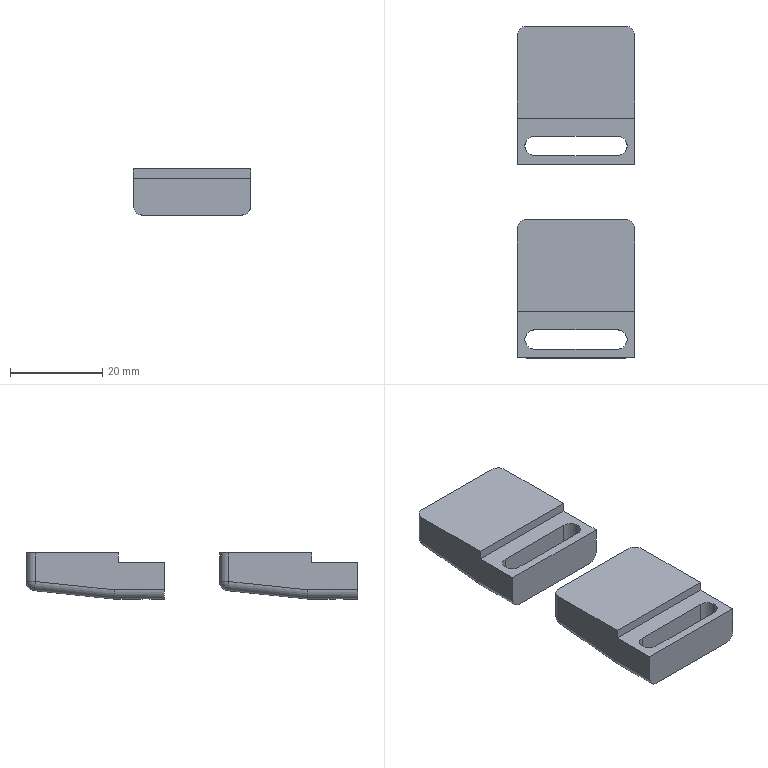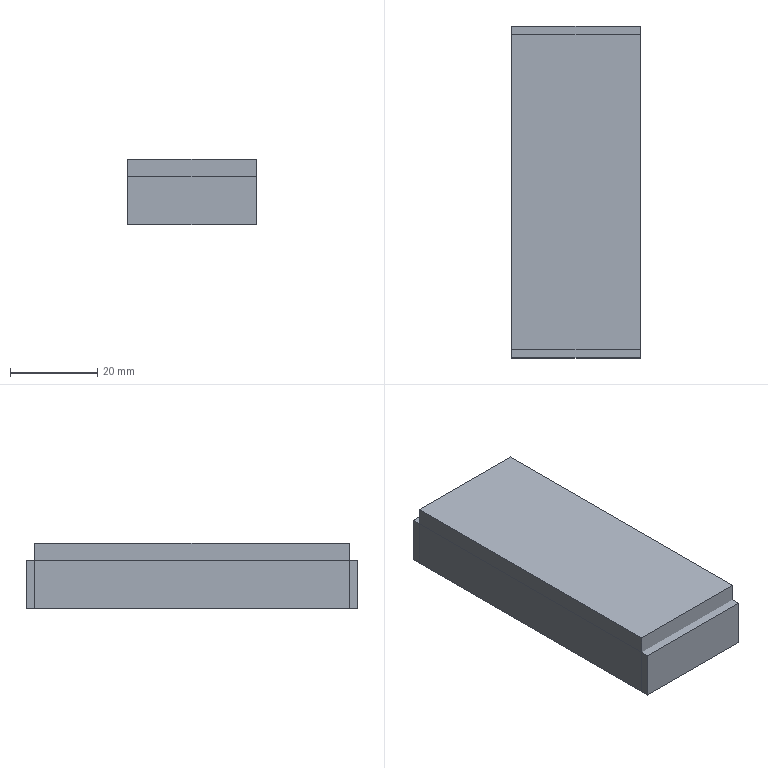CAM job | NX | 3+2 milling | part box 25.5 x 72 x 10 mm | stock box 29.5 x 76 x 15 mm
Tools:
number,name,description,diameter,corner_radius,flute_length,length,flutes
19,D80,Milling Tool-5 Parameters,80.0,0.0,50.0,75.0,2
14,D10JING,Milling Tool-5 Parameters,10.0,0.0,50.0,75.0,2
15,D10,Milling Tool-5 Parameters,10.0,0.0,50.0,75.0,2
12,D6,Milling Tool-5 Parameters,6.0,0.0,50.0,75.0,2
17,D3,Milling Tool-5 Parameters,3.0,0.0,50.0,75.0,2
1,D6A45,Milling Tool-5 Parameters,6.0,0.0,50.0,75.0,2
16,D4R0.5,Milling Tool-5 Parameters,4.0,0.5,50.0,75.0,2
18,R2,Milling Tool-5 Parameters,4.0,2.0,50.0,75.0,2
Operations:
program,operation,operation_type,tool,method,geometry_group,spindle_rpm,surface_speed,feed_per_tooth,feed_cut,feed_plunge,cut_length_mm,path_length_mm,cut_time_min,machine_time_min
1,FLOOR_WALL_COPY,VolumeBased25DMillingOperation,D80,METHOD,A,6500.0,1633.0,0.1154,1500.0,100.0,172.0,226.0,0.1147,0.1201
1,ZLEVEL_PROFILE,ZLevelMilling,D10,METHOD,A,9500.0,298.0,0.1579,3000.0,1000.0,3039.798,3291.531,1.077,1.102
1,FLOOR_WALL,VolumeBased25DMillingOperation,D10,METHOD,A,9500.0,298.0,0.1316,2500.0,1000.0,621.396,804.327,0.2562,0.2745
1,ZLEVEL_PROFILE_COPY_1_COPY_COPY_1,ZLevelMilling,D10JING,METHOD,A,9500.0,298.0,0.0632,1200.0,1000.0,296.075,497.43,0.2479,0.2681
1,FLOOR_WALL_1,VolumeBased25DMillingOperation,D10JING,METHOD,A,9500.0,119.0,0.0658,1250.0,100.0,401.873,734.258,0.3215,0.3547
1,ZLEVEL_PROFILE_COPY,ZLevelMilling,D3,METHOD,A,9500.0,89.0,0.0632,1200.0,1000.0,2253.304,2434.812,1.889,1.907
1,PLANAR_MILL_COPY_COPY_COPY_COPY_COPY_COPY_1_COPY_1,PlanarMilling,D6A45,METHOD,A,9500.0,179.0,0.0658,1250.0,100.0,200.065,382.865,0.1601,0.1783
1,PLANAR_MILL_COPY_COPY_COPY_COPY_COPY_COPY_1_COPY_1_COPY,PlanarMilling,D6A45,METHOD,A,9500.0,179.0,0.0658,1250.0,100.0,196.179,530.234,0.1569,0.1903
2,FLOOR_WALL_COPY_COPY,VolumeBased25DMillingOperation,D80,METHOD,B,6500.0,1633.0,0.1154,1500.0,100.0,860.0,1774.001,0.5733,0.6647
2,PLANAR_MILL_COPY_COPY_COPY_COPY_COPY_COPY_1_COPY_1_COPY_1,PlanarMilling,D6A45,METHOD,B,9500.0,179.0,0.0658,1250.0,100.0,97.268,258.668,0.0778,0.094
2,FIXED_CONTOUR,SurfaceContour,D4R0.5,METHOD,B,9500.0,119.0,0.1316,2500.0,1000.0,20865.772,21474.38,8.408,8.469
2,FIXED_CONTOUR_COPY,SurfaceContour,R2,METHOD,B,9500.0,119.0,0.1316,2500.0,1000.0,2996.156,3134.2,1.204,1.218
3,HOLE_MILLING,CylinderMilling,D6,METHOD,C,9500.0,298.0,0.0658,1250.0,100.0,277.274,356.774,0.2218,0.2298